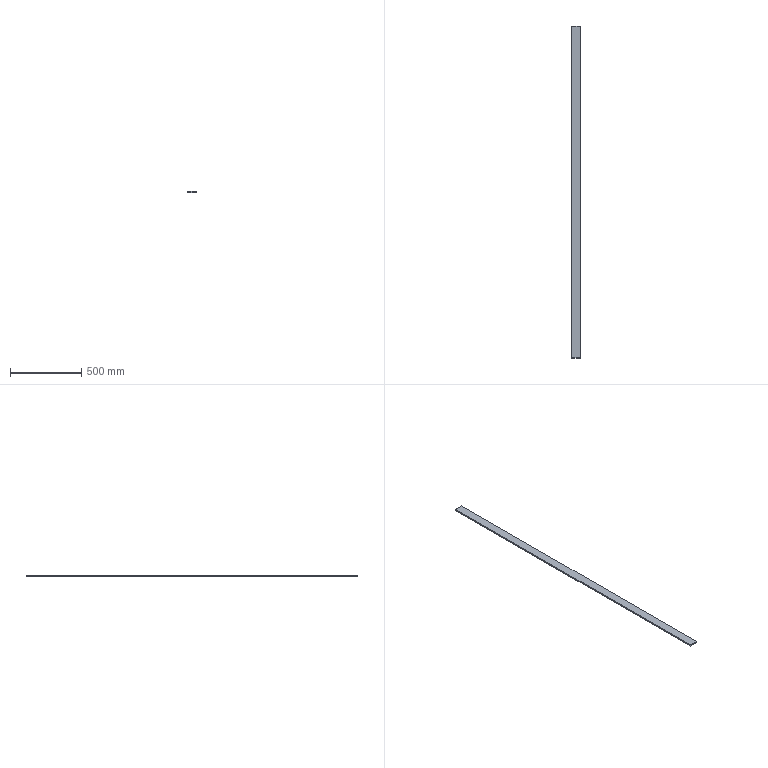Part | SolidWorks | features Extrusion 1 | 1 solid | 6 faces | box 60 x 2330 x 10 mm | volume 1398000 mm3 | plane 6
STEP:
#1=CARTESIAN_POINT('',(0.,2330.,0.));
#2=VERTEX_POINT('',#1);
#3=CARTESIAN_POINT('',(0.,0.,0.));
#4=VERTEX_POINT('',#3);
#5=CARTESIAN_POINT('',(0.,0.,0.));
#6=DIRECTION('',(0.,-1.,0.));
#7=VECTOR('',#6,1000.);
#8=LINE('',#5,#7);
#9=EDGE_CURVE('',#2,#4,#8,.T.);
#10=ORIENTED_EDGE('',*,*,#9,.T.);
#11=CARTESIAN_POINT('',(0.,0.,10.));
#12=VERTEX_POINT('',#11);
#13=CARTESIAN_POINT('',(0.,0.,10.));
#14=DIRECTION('',(0.,0.,-1.));
#15=VECTOR('',#14,1000.);
#16=LINE('',#13,#15);
#17=EDGE_CURVE('',#12,#4,#16,.T.);
#18=ORIENTED_EDGE('',*,*,#17,.F.);
#19=CARTESIAN_POINT('',(0.,2330.,10.));
#20=VERTEX_POINT('',#19);
#21=CARTESIAN_POINT('',(0.,0.,10.));
#22=DIRECTION('',(0.,-1.,0.));
#23=VECTOR('',#22,1000.);
#24=LINE('',#21,#23);
#25=EDGE_CURVE('',#20,#12,#24,.T.);
#26=ORIENTED_EDGE('',*,*,#25,.F.);
#27=CARTESIAN_POINT('',(0.,2330.,10.));
#28=DIRECTION('',(0.,0.,-1.));
#29=VECTOR('',#28,1000.);
#30=LINE('',#27,#29);
#31=EDGE_CURVE('',#20,#2,#30,.T.);
#32=ORIENTED_EDGE('',*,*,#31,.T.);
#33=EDGE_LOOP('',(#10,#18,#26,#32));
#34=FACE_OUTER_BOUND('',#33,.T.);
#35=CARTESIAN_POINT('',(0.,0.,10.));
#36=DIRECTION('',(1.,0.,0.));
#37=DIRECTION('',(0.,1.,0.));
#38=AXIS2_PLACEMENT_3D('',#35,#36,#37);
#39=PLANE('',#38);
#40=ADVANCED_FACE('',(#34),#39,.F.);
#41=CARTESIAN_POINT('',(60.,0.,0.));
#42=VERTEX_POINT('',#41);
#43=CARTESIAN_POINT('',(0.,0.,0.));
#44=DIRECTION('',(1.,0.,0.));
#45=VECTOR('',#44,1000.);
#46=LINE('',#43,#45);
#47=EDGE_CURVE('',#4,#42,#46,.T.);
#48=ORIENTED_EDGE('',*,*,#47,.T.);
#49=CARTESIAN_POINT('',(60.,0.,10.));
#50=VERTEX_POINT('',#49);
#51=CARTESIAN_POINT('',(60.,0.,10.));
#52=DIRECTION('',(0.,0.,-1.));
#53=VECTOR('',#52,1000.);
#54=LINE('',#51,#53);
#55=EDGE_CURVE('',#50,#42,#54,.T.);
#56=ORIENTED_EDGE('',*,*,#55,.F.);
#57=CARTESIAN_POINT('',(0.,0.,10.));
#58=DIRECTION('',(1.,0.,0.));
#59=VECTOR('',#58,1000.);
#60=LINE('',#57,#59);
#61=EDGE_CURVE('',#12,#50,#60,.T.);
#62=ORIENTED_EDGE('',*,*,#61,.F.);
#63=ORIENTED_EDGE('',*,*,#17,.T.);
#64=EDGE_LOOP('',(#48,#56,#62,#63));
#65=FACE_OUTER_BOUND('',#64,.T.);
#66=CARTESIAN_POINT('',(0.,0.,10.));
#67=DIRECTION('',(0.,1.,0.));
#68=DIRECTION('',(0.,0.,1.));
#69=AXIS2_PLACEMENT_3D('',#66,#67,#68);
#70=PLANE('',#69);
#71=ADVANCED_FACE('',(#65),#70,.F.);
#72=CARTESIAN_POINT('',(60.,2330.,0.));
#73=VERTEX_POINT('',#72);
#74=CARTESIAN_POINT('',(60.,0.,0.));
#75=DIRECTION('',(0.,1.,0.));
#76=VECTOR('',#75,1000.);
#77=LINE('',#74,#76);
#78=EDGE_CURVE('',#42,#73,#77,.T.);
#79=ORIENTED_EDGE('',*,*,#78,.T.);
#80=CARTESIAN_POINT('',(60.,2330.,10.));
#81=VERTEX_POINT('',#80);
#82=CARTESIAN_POINT('',(60.,2330.,10.));
#83=DIRECTION('',(0.,0.,-1.));
#84=VECTOR('',#83,1000.);
#85=LINE('',#82,#84);
#86=EDGE_CURVE('',#81,#73,#85,.T.);
#87=ORIENTED_EDGE('',*,*,#86,.F.);
#88=CARTESIAN_POINT('',(60.,0.,10.));
#89=DIRECTION('',(0.,1.,0.));
#90=VECTOR('',#89,1000.);
#91=LINE('',#88,#90);
#92=EDGE_CURVE('',#50,#81,#91,.T.);
#93=ORIENTED_EDGE('',*,*,#92,.F.);
#94=ORIENTED_EDGE('',*,*,#55,.T.);
#95=EDGE_LOOP('',(#79,#87,#93,#94));
#96=FACE_OUTER_BOUND('',#95,.T.);
#97=CARTESIAN_POINT('',(60.,0.,10.));
#98=DIRECTION('',(-1.,0.,0.));
#99=DIRECTION('',(0.,-1.,0.));
#100=AXIS2_PLACEMENT_3D('',#97,#98,#99);
#101=PLANE('',#100);
#102=ADVANCED_FACE('',(#96),#101,.F.);
#103=CARTESIAN_POINT('',(0.,2330.,0.));
#104=DIRECTION('',(-1.,0.,0.));
#105=VECTOR('',#104,1000.);
#106=LINE('',#103,#105);
#107=EDGE_CURVE('',#73,#2,#106,.T.);
#108=ORIENTED_EDGE('',*,*,#107,.T.);
#109=ORIENTED_EDGE('',*,*,#31,.F.);
#110=CARTESIAN_POINT('',(0.,2330.,10.));
#111=DIRECTION('',(-1.,0.,0.));
#112=VECTOR('',#111,1000.);
#113=LINE('',#110,#112);
#114=EDGE_CURVE('',#81,#20,#113,.T.);
#115=ORIENTED_EDGE('',*,*,#114,.F.);
#116=ORIENTED_EDGE('',*,*,#86,.T.);
#117=EDGE_LOOP('',(#108,#109,#115,#116));
#118=FACE_OUTER_BOUND('',#117,.T.);
#119=CARTESIAN_POINT('',(0.,2330.,10.));
#120=DIRECTION('',(0.,-1.,0.));
#121=DIRECTION('',(0.,0.,-1.));
#122=AXIS2_PLACEMENT_3D('',#119,#120,#121);
#123=PLANE('',#122);
#124=ADVANCED_FACE('',(#118),#123,.F.);
#125=ORIENTED_EDGE('',*,*,#25,.T.);
#126=ORIENTED_EDGE('',*,*,#61,.T.);
#127=ORIENTED_EDGE('',*,*,#92,.T.);
#128=ORIENTED_EDGE('',*,*,#114,.T.);
#129=EDGE_LOOP('',(#125,#126,#127,#128));
#130=FACE_OUTER_BOUND('',#129,.T.);
#131=CARTESIAN_POINT('',(0.,0.,10.));
#132=DIRECTION('',(0.,0.,-1.));
#133=DIRECTION('',(-1.,0.,0.));
#134=AXIS2_PLACEMENT_3D('',#131,#132,#133);
#135=PLANE('',#134);
#136=ADVANCED_FACE('',(#130),#135,.F.);
#137=ORIENTED_EDGE('',*,*,#9,.F.);
#138=ORIENTED_EDGE('',*,*,#107,.F.);
#139=ORIENTED_EDGE('',*,*,#78,.F.);
#140=ORIENTED_EDGE('',*,*,#47,.F.);
#141=EDGE_LOOP('',(#137,#138,#139,#140));
#142=FACE_OUTER_BOUND('',#141,.T.);
#143=CARTESIAN_POINT('',(0.,0.,0.));
#144=DIRECTION('',(0.,0.,-1.));
#145=DIRECTION('',(-1.,0.,0.));
#146=AXIS2_PLACEMENT_3D('',#143,#144,#145);
#147=PLANE('',#146);
#148=ADVANCED_FACE('',(#142),#147,.T.);
#149=CLOSED_SHELL('',(#40,#71,#102,#124,#136,#148));
#150=MANIFOLD_SOLID_BREP('',#149);
#151=CARTESIAN_POINT('',(0.,0.,0.));
#152=DIRECTION('',(0.,0.,1.));
#153=DIRECTION('',(1.,0.,0.));
#154=AXIS2_PLACEMENT_3D('',#151,#152,#153);
#155=(LENGTH_UNIT()NAMED_UNIT(*)SI_UNIT(.MILLI.,.METRE.));
#156=UNCERTAINTY_MEASURE_WITH_UNIT(LENGTH_MEASURE(0.00001),#155,'','');
#157=(NAMED_UNIT(*)PLANE_ANGLE_UNIT()SI_UNIT($,.RADIAN.));
#158=(NAMED_UNIT(*)SI_UNIT($,.STERADIAN.)SOLID_ANGLE_UNIT());
#159=(GEOMETRIC_REPRESENTATION_CONTEXT(3)GLOBAL_UNCERTAINTY_ASSIGNED_CONTEXT((#156))GLOBAL_UNIT_ASSIGNED_CONTEXT((#155,#157,#158))REPRESENTATION_CONTEXT('',''));
#160=ADVANCED_BREP_SHAPE_REPRESENTATION('',(#150,#154),#159);